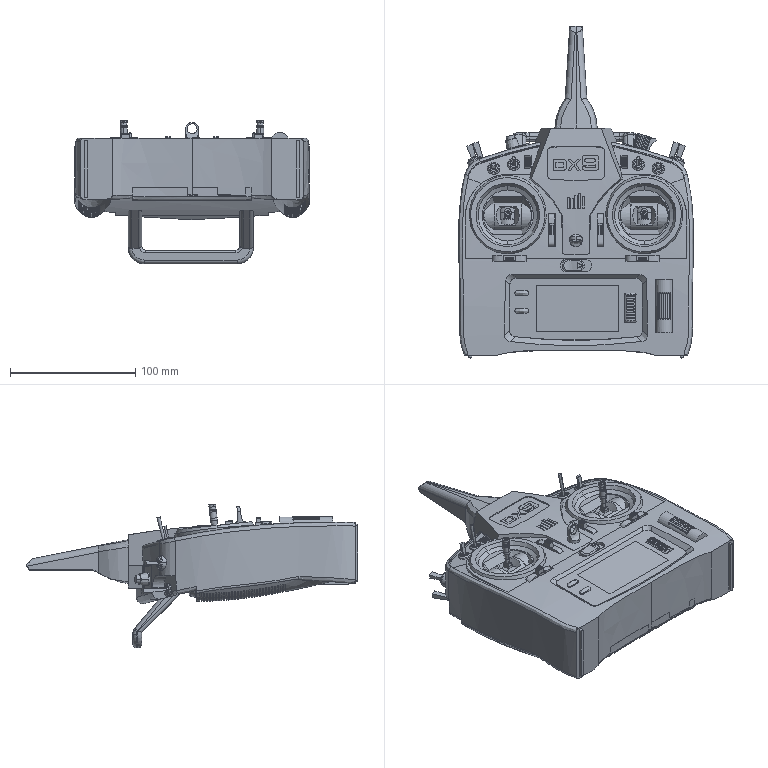Part | SolidWorks | features BaseBody 5 | 5 solids | 1783 faces | box 187.605 x 265.079 x 114.815 mm | volume 1499845 mm3 | plane 1215 | cylinder 341 | spline 148 | cone 52 | torus 23 | sphere 4 | commonest cylinder face diameters 1.04 x39 1.302 x24 2 x23 4 x23 10 x19 2.4 x16